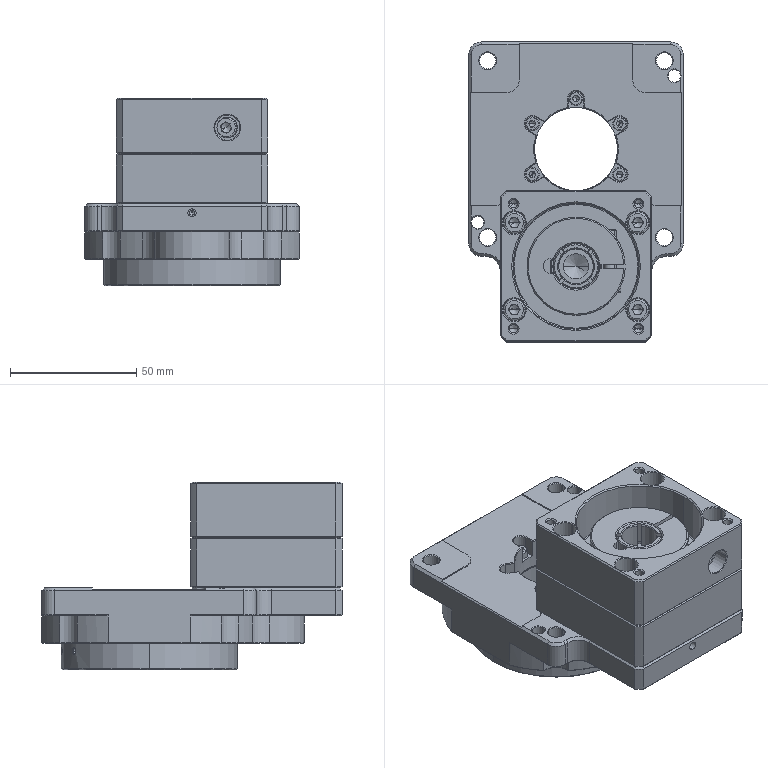Part | SolidWorks | 33 solids | 1768 faces | box 85 x 119 x 74.5 mm | volume 264146 mm3 | plane 532 | cone 466 | cylinder 389 | torus 225 | sphere 152 | spline 4 | commonest cylinder face diameters 5 x28 5.5 x28 3 x26 3.5 x24 3.3 x22 8.5 x18